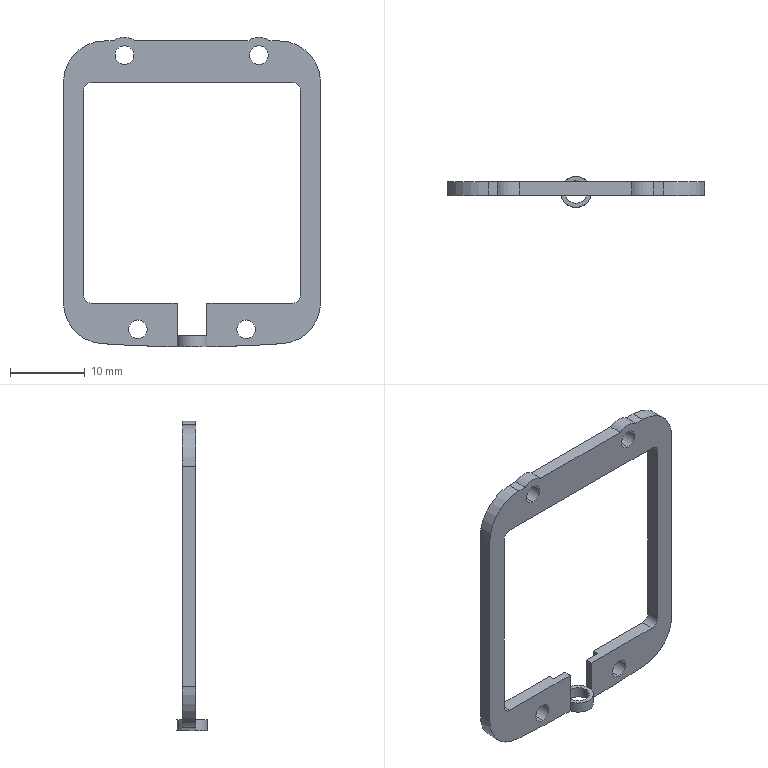Part | SolidWorks | features ICE 5, Extrusion 1 | 1 solid | 43 faces | box 34.4 x 4.123 x 41.42 mm | volume 850.585 mm3 | cylinder 24 | plane 19 | commonest cylinder face diameters 2.5 x8 2 x4 11 x4 3 x2 4.123 x2 4.8 x2